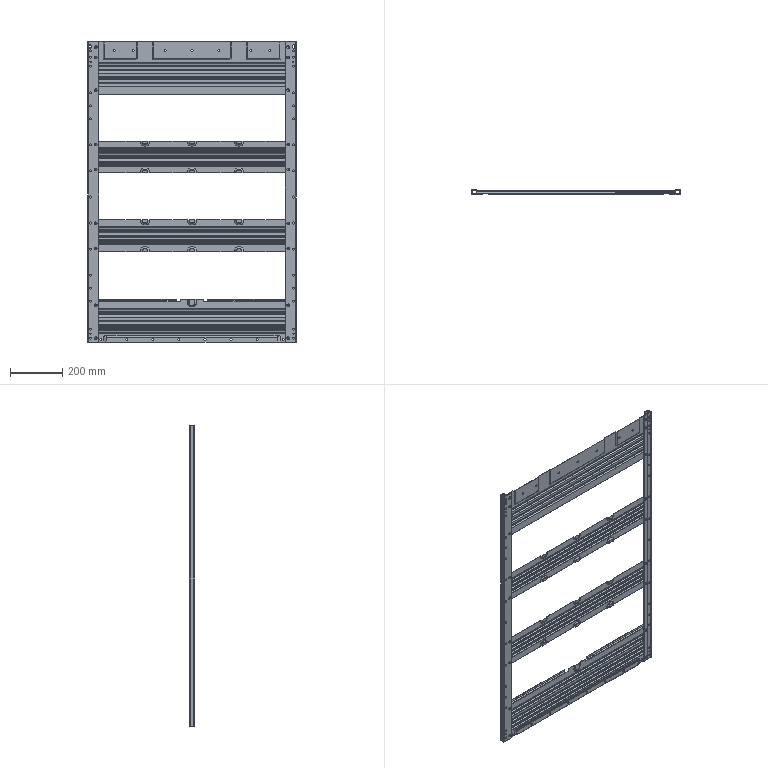Part | NX | features BREP 5 | 6 solids | 1175 faces | box 800.596 x 20.401 x 1150 mm | volume 1198428 mm3 | plane 586 | cylinder 385 | torus 104 | cone 92 | spline 4 | sphere 4 | commonest cylinder face diameters 5.1 x72 6 x44 2 x41 4.4 x41 3.6 x39 10 x31